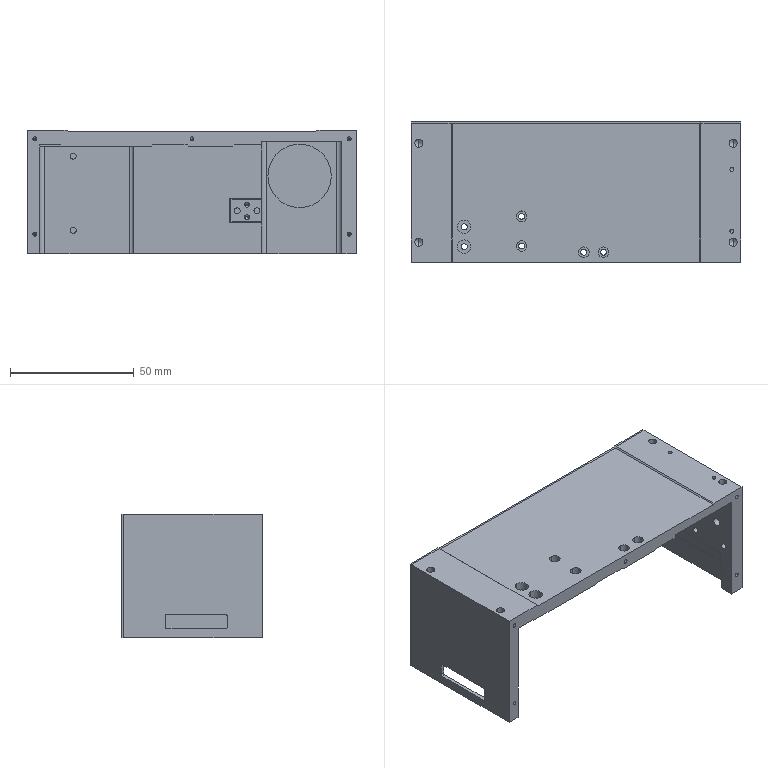NC program | NX | posted with a generic post | part box 133 x 56.74 x 50 mm
Whole program:
N10 G17 G21 G94 G90
(DRILLING_COPY_1_COPY_COPY_1 , TOOL : D6A45)
N12 T07 M6
N14 G54
N16 G17 G0 G90 X63.5 Y-3.5 B0. C0. S5000 M3
N18 G43 Z30. H7
N20 G94 G81 G98 Z-1. F250. R3.
N22 Y-42.
N24 X-63.5
N26 Y-3.5
N28 X0.
N30 X22.25 Y-30.14 Z-50.5 R-46.5
N32 Y-35.14
N34 G80
N36 G0 X22.25 Y-35.14 Z30.
N38 M5
(DRILLING_COPY_COPY_COPY_1_COPY , TOOL : 1.6ZT)
N40 T14 M6
N42 G54
N44 G17 G0 G90 X63.5 Y-3.5 B0. C0. S2000 M3
N46 G43 Z30. H14
N48 G94 G83 G98 Z-5.2 F150. Q2. R3.
N50 Y-42.
N52 X-63.5
N54 Y-3.5
N56 X0.
N58 G80
N60 G0 X0. Y-3.5 Z30.
N62 M5
(PLANAR_MILL_1 , TOOL : D10JING)
N64 T09 M6
N66 G54
N68 G17 G0 G90 X14.75 Y-17.616 B0. C0. S8000 M3
N70 G43 Z30. H9
N72 Z-48.35
N74 G94 G1 Z-49.85 F1250.
N76 G3 X15.25 Y-16.75 R1.
N78 G1 Y-11.
N80 X28.25
N82 Y-22.5
N84 X15.25
N86 Y-16.75
N88 X20.25
N90 Y-16.
N92 X23.25
N94 Y-17.5
N96 X20.25
N98 Y-16.75
N100 G3 X19.75 Y-15.884 R1.
N102 G1 Z-48.35
N104 G0 X14.75 Y-17.616 Z-48.5
N106 G1 Z-50.
N108 G3 X15.25 Y-16.75 R1.
N110 G1 Y-11.
N112 X28.25
N114 Y-22.5
N116 X15.25
N118 Y-16.75
N120 X20.25
N122 Y-16.
N124 X23.25
N126 Y-17.5
N128 X20.25
N130 Y-16.75
N132 G3 X19.75 Y-15.884 R1.
N134 G1 Z-48.5
N136 G0 Z30.
N138 M5
N140 M2